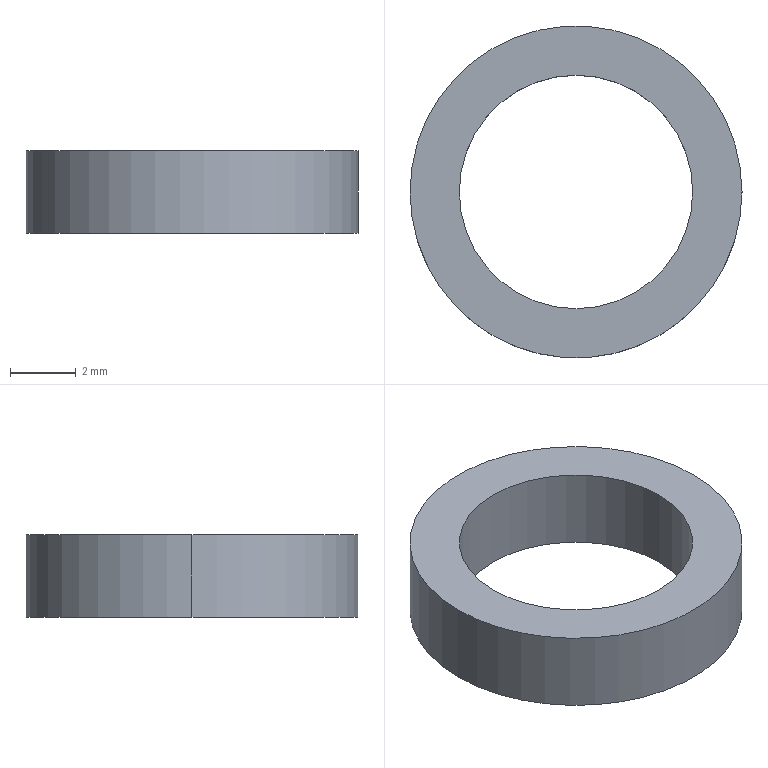Part | NX | features BREP 1 | 1 solid | 6 faces | box 10.1 x 10.1 x 2.5 mm | volume 101.316 mm3 | cylinder 4 | plane 2 | commonest cylinder face diameters 7.1 x2 10.1 x2
STEP:
#1=CARTESIAN_POINT('',(3.55,0.,2.5));
#2=VERTEX_POINT('',#1);
#3=CARTESIAN_POINT('',(3.55,0.,0.));
#4=VERTEX_POINT('',#3);
#5=CARTESIAN_POINT('',(3.55,0.,2.5));
#6=DIRECTION('',(0.,0.,-1.));
#7=VECTOR('',#6,1000.);
#8=LINE('',#5,#7);
#9=EDGE_CURVE('',#2,#4,#8,.T.);
#10=ORIENTED_EDGE('',*,*,#9,.F.);
#11=CARTESIAN_POINT('',(-3.55,0.,2.5));
#12=VERTEX_POINT('',#11);
#13=CARTESIAN_POINT('',(0.,0.,2.5));
#14=DIRECTION('',(0.,0.,1.));
#15=DIRECTION('',(1.,0.,0.));
#16=AXIS2_PLACEMENT_3D('',#13,#14,#15);
#17=CIRCLE('',#16,3.55);
#18=EDGE_CURVE('',#2,#12,#17,.T.);
#19=ORIENTED_EDGE('',*,*,#18,.T.);
#20=CARTESIAN_POINT('',(-3.55,0.,0.));
#21=VERTEX_POINT('',#20);
#22=CARTESIAN_POINT('',(-3.55,0.,2.5));
#23=DIRECTION('',(0.,0.,-1.));
#24=VECTOR('',#23,1000.);
#25=LINE('',#22,#24);
#26=EDGE_CURVE('',#12,#21,#25,.T.);
#27=ORIENTED_EDGE('',*,*,#26,.T.);
#28=CARTESIAN_POINT('',(0.,0.,0.));
#29=DIRECTION('',(0.,0.,1.));
#30=DIRECTION('',(1.,0.,0.));
#31=AXIS2_PLACEMENT_3D('',#28,#29,#30);
#32=CIRCLE('',#31,3.55);
#33=EDGE_CURVE('',#4,#21,#32,.T.);
#34=ORIENTED_EDGE('',*,*,#33,.F.);
#35=EDGE_LOOP('',(#10,#19,#27,#34));
#36=FACE_BOUND('',#35,.T.);
#37=CARTESIAN_POINT('',(0.,0.,2.5));
#38=DIRECTION('',(0.,0.,-1.));
#39=DIRECTION('',(-1.,0.,0.));
#40=AXIS2_PLACEMENT_3D('',#37,#38,#39);
#41=CYLINDRICAL_SURFACE('',#40,3.55);
#42=ADVANCED_FACE('',(#36),#41,.F.);
#43=CARTESIAN_POINT('',(5.05,0.,2.5));
#44=VERTEX_POINT('',#43);
#45=CARTESIAN_POINT('',(5.05,0.,0.));
#46=VERTEX_POINT('',#45);
#47=CARTESIAN_POINT('',(5.05,0.,2.5));
#48=DIRECTION('',(0.,0.,-1.));
#49=VECTOR('',#48,1000.);
#50=LINE('',#47,#49);
#51=EDGE_CURVE('',#44,#46,#50,.T.);
#52=ORIENTED_EDGE('',*,*,#51,.F.);
#53=CARTESIAN_POINT('',(-5.05,0.,2.5));
#54=VERTEX_POINT('',#53);
#55=CARTESIAN_POINT('',(0.,0.,2.5));
#56=DIRECTION('',(0.,0.,1.));
#57=DIRECTION('',(1.,0.,0.));
#58=AXIS2_PLACEMENT_3D('',#55,#56,#57);
#59=CIRCLE('',#58,5.05);
#60=EDGE_CURVE('',#54,#44,#59,.T.);
#61=ORIENTED_EDGE('',*,*,#60,.F.);
#62=CARTESIAN_POINT('',(-5.05,0.,0.));
#63=VERTEX_POINT('',#62);
#64=CARTESIAN_POINT('',(-5.05,0.,2.5));
#65=DIRECTION('',(0.,0.,-1.));
#66=VECTOR('',#65,1000.);
#67=LINE('',#64,#66);
#68=EDGE_CURVE('',#54,#63,#67,.T.);
#69=ORIENTED_EDGE('',*,*,#68,.T.);
#70=CARTESIAN_POINT('',(0.,0.,0.));
#71=DIRECTION('',(0.,0.,1.));
#72=DIRECTION('',(1.,0.,0.));
#73=AXIS2_PLACEMENT_3D('',#70,#71,#72);
#74=CIRCLE('',#73,5.05);
#75=EDGE_CURVE('',#63,#46,#74,.T.);
#76=ORIENTED_EDGE('',*,*,#75,.T.);
#77=EDGE_LOOP('',(#52,#61,#69,#76));
#78=FACE_BOUND('',#77,.T.);
#79=CARTESIAN_POINT('',(0.,0.,2.5));
#80=DIRECTION('',(0.,0.,-1.));
#81=DIRECTION('',(-1.,0.,0.));
#82=AXIS2_PLACEMENT_3D('',#79,#80,#81);
#83=CYLINDRICAL_SURFACE('',#82,5.05);
#84=ADVANCED_FACE('',(#78),#83,.T.);
#85=CARTESIAN_POINT('',(0.,0.,0.));
#86=DIRECTION('',(0.,0.,1.));
#87=DIRECTION('',(1.,0.,0.));
#88=AXIS2_PLACEMENT_3D('',#85,#86,#87);
#89=CIRCLE('',#88,3.55);
#90=EDGE_CURVE('',#21,#4,#89,.T.);
#91=ORIENTED_EDGE('',*,*,#90,.T.);
#92=ORIENTED_EDGE('',*,*,#33,.T.);
#93=EDGE_LOOP('',(#91,#92));
#94=FACE_BOUND('',#93,.T.);
#95=ORIENTED_EDGE('',*,*,#75,.F.);
#96=CARTESIAN_POINT('',(0.,0.,0.));
#97=DIRECTION('',(0.,0.,1.));
#98=DIRECTION('',(1.,0.,0.));
#99=AXIS2_PLACEMENT_3D('',#96,#97,#98);
#100=CIRCLE('',#99,5.05);
#101=EDGE_CURVE('',#46,#63,#100,.T.);
#102=ORIENTED_EDGE('',*,*,#101,.F.);
#103=EDGE_LOOP('',(#95,#102));
#104=FACE_BOUND('',#103,.T.);
#105=CARTESIAN_POINT('',(0.,0.,0.));
#106=DIRECTION('',(0.,0.,1.));
#107=DIRECTION('',(1.,0.,0.));
#108=AXIS2_PLACEMENT_3D('',#105,#106,#107);
#109=PLANE('',#108);
#110=ADVANCED_FACE('',(#94,#104),#109,.F.);
#111=CARTESIAN_POINT('',(0.,0.,2.5));
#112=DIRECTION('',(0.,0.,1.));
#113=DIRECTION('',(1.,0.,0.));
#114=AXIS2_PLACEMENT_3D('',#111,#112,#113);
#115=CIRCLE('',#114,3.55);
#116=EDGE_CURVE('',#12,#2,#115,.T.);
#117=ORIENTED_EDGE('',*,*,#116,.F.);
#118=ORIENTED_EDGE('',*,*,#18,.F.);
#119=EDGE_LOOP('',(#117,#118));
#120=FACE_BOUND('',#119,.T.);
#121=ORIENTED_EDGE('',*,*,#60,.T.);
#122=CARTESIAN_POINT('',(0.,0.,2.5));
#123=DIRECTION('',(0.,0.,1.));
#124=DIRECTION('',(1.,0.,0.));
#125=AXIS2_PLACEMENT_3D('',#122,#123,#124);
#126=CIRCLE('',#125,5.05);
#127=EDGE_CURVE('',#44,#54,#126,.T.);
#128=ORIENTED_EDGE('',*,*,#127,.T.);
#129=EDGE_LOOP('',(#121,#128));
#130=FACE_BOUND('',#129,.T.);
#131=CARTESIAN_POINT('',(0.,0.,2.5));
#132=DIRECTION('',(0.,0.,1.));
#133=DIRECTION('',(1.,0.,0.));
#134=AXIS2_PLACEMENT_3D('',#131,#132,#133);
#135=PLANE('',#134);
#136=ADVANCED_FACE('',(#120,#130),#135,.T.);
#137=ORIENTED_EDGE('',*,*,#127,.F.);
#138=ORIENTED_EDGE('',*,*,#51,.T.);
#139=ORIENTED_EDGE('',*,*,#101,.T.);
#140=ORIENTED_EDGE('',*,*,#68,.F.);
#141=EDGE_LOOP('',(#137,#138,#139,#140));
#142=FACE_BOUND('',#141,.T.);
#143=CARTESIAN_POINT('',(0.,0.,2.5));
#144=DIRECTION('',(0.,0.,-1.));
#145=DIRECTION('',(-1.,0.,0.));
#146=AXIS2_PLACEMENT_3D('',#143,#144,#145);
#147=CYLINDRICAL_SURFACE('',#146,5.05);
#148=ADVANCED_FACE('',(#142),#147,.T.);
#149=ORIENTED_EDGE('',*,*,#116,.T.);
#150=ORIENTED_EDGE('',*,*,#9,.T.);
#151=ORIENTED_EDGE('',*,*,#90,.F.);
#152=ORIENTED_EDGE('',*,*,#26,.F.);
#153=EDGE_LOOP('',(#149,#150,#151,#152));
#154=FACE_BOUND('',#153,.T.);
#155=CARTESIAN_POINT('',(0.,0.,2.5));
#156=DIRECTION('',(0.,0.,-1.));
#157=DIRECTION('',(-1.,0.,0.));
#158=AXIS2_PLACEMENT_3D('',#155,#156,#157);
#159=CYLINDRICAL_SURFACE('',#158,3.55);
#160=ADVANCED_FACE('',(#154),#159,.F.);
#161=CLOSED_SHELL('',(#42,#84,#110,#136,#148,#160));
#162=MANIFOLD_SOLID_BREP('',#161);
#163=(LENGTH_UNIT()NAMED_UNIT(*)SI_UNIT(.MILLI.,.METRE.));
#164=UNCERTAINTY_MEASURE_WITH_UNIT(LENGTH_MEASURE(0.00001),#163,'','');
#165=(NAMED_UNIT(*)PLANE_ANGLE_UNIT()SI_UNIT($,.RADIAN.));
#166=(NAMED_UNIT(*)SI_UNIT($,.STERADIAN.)SOLID_ANGLE_UNIT());
#167=(GEOMETRIC_REPRESENTATION_CONTEXT(3)GLOBAL_UNCERTAINTY_ASSIGNED_CONTEXT((#164))GLOBAL_UNIT_ASSIGNED_CONTEXT((#163,#165,#166))REPRESENTATION_CONTEXT('',''));
#168=ADVANCED_BREP_SHAPE_REPRESENTATION('',(#162),#167);